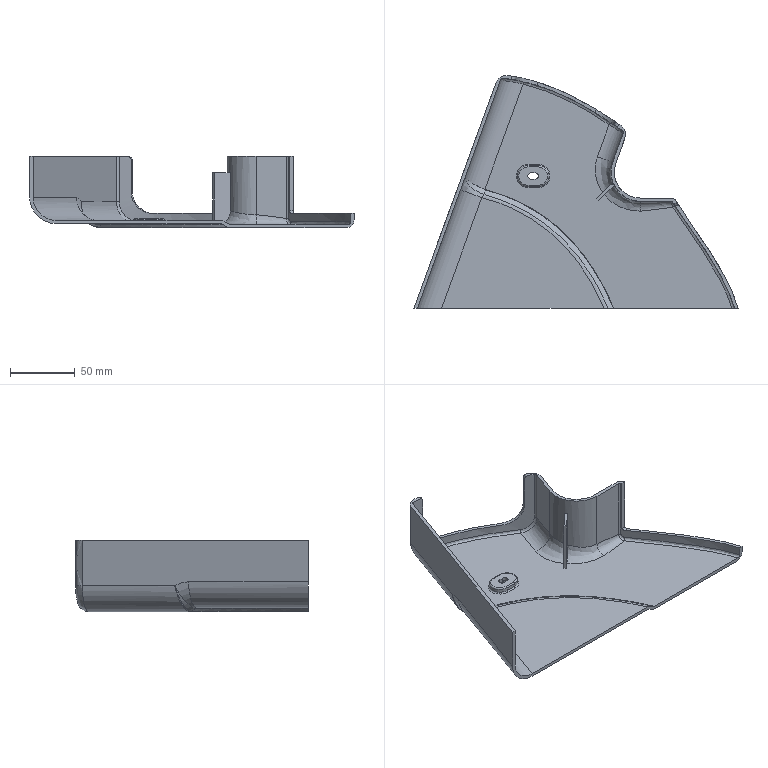Part | STEP file | LZHT-R1 | 1 solid | 102 faces | box 250 x 180.091 x 55 mm | volume 106562 mm3 | spline 40 | plane 30 | cylinder 26 | torus 6 | commonest cylinder face diameters 2 x6 4 x4 40 x3 5 x2 6 x2 10 x2